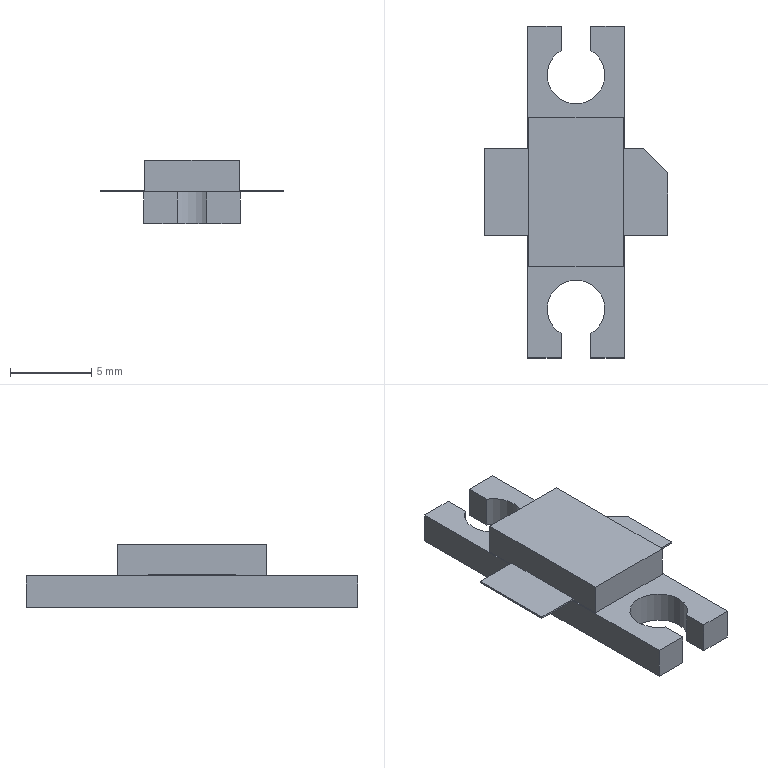Part | STEP file | YP40601625T | 1 solid | 31 faces | box 11.3 x 20.43 x 3.88 mm | volume 294.314 mm3 | plane 29 | cylinder 2 | commonest cylinder face diameters 3.55 x2